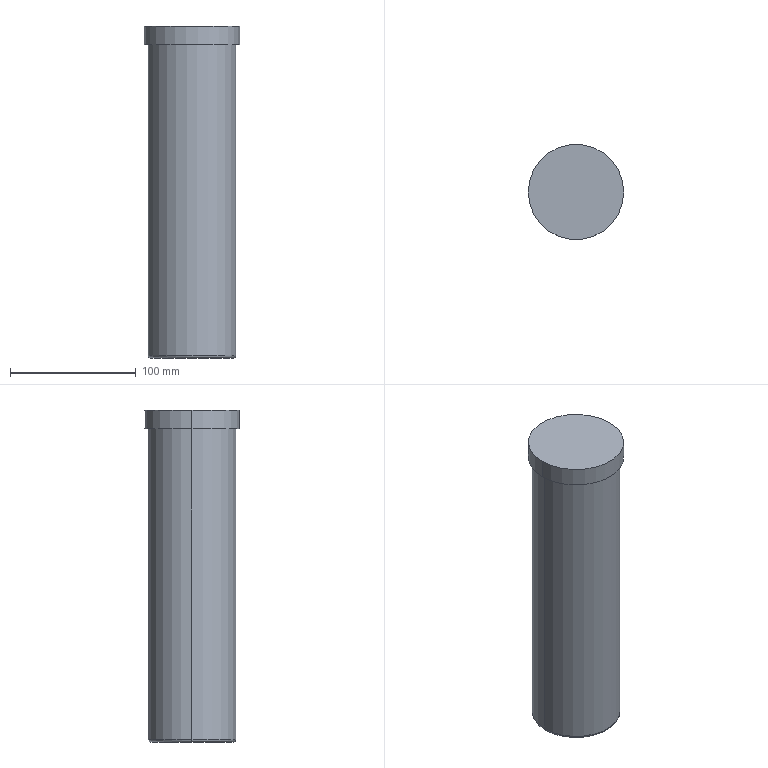Part | SolidWorks | features BaseBody 1 | 1 solid | 9 faces | box 76 x 76 x 264.5 mm | volume 1028049 mm3 | cylinder 4 | plane 3 | torus 2 | commonest cylinder face diameters 70 x2 76 x2
STEP:
#1=CARTESIAN_POINT('',(-378.,-275.,-94.));
#2=VERTEX_POINT('',#1);
#3=CARTESIAN_POINT('',(-312.,-275.,-94.));
#4=VERTEX_POINT('',#3);
#5=CARTESIAN_POINT('',(-345.,-275.,-94.));
#6=DIRECTION('',(0.,0.,-1.));
#7=DIRECTION('',(1.,0.,0.));
#8=AXIS2_PLACEMENT_3D('',#5,#6,#7);
#9=CIRCLE('',#8,33.);
#10=EDGE_CURVE('',#2,#4,#9,.T.);
#11=ORIENTED_EDGE('',*,*,#10,.F.);
#12=CARTESIAN_POINT('',(-380.,-275.,-92.));
#13=VERTEX_POINT('',#12);
#14=CARTESIAN_POINT('',(-378.,-275.,-92.));
#15=DIRECTION('',(0.,1.,0.));
#16=DIRECTION('',(-1.,0.,0.));
#17=AXIS2_PLACEMENT_3D('',#14,#15,#16);
#18=CIRCLE('',#17,2.);
#19=EDGE_CURVE('',#2,#13,#18,.T.);
#20=ORIENTED_EDGE('',*,*,#19,.T.);
#21=CARTESIAN_POINT('',(-310.,-275.,-92.));
#22=VERTEX_POINT('',#21);
#23=CARTESIAN_POINT('',(-345.,-275.,-92.));
#24=DIRECTION('',(0.,0.,1.));
#25=DIRECTION('',(1.,0.,0.));
#26=AXIS2_PLACEMENT_3D('',#23,#24,#25);
#27=CIRCLE('',#26,35.);
#28=EDGE_CURVE('',#22,#13,#27,.T.);
#29=ORIENTED_EDGE('',*,*,#28,.F.);
#30=CARTESIAN_POINT('',(-312.,-275.,-92.));
#31=DIRECTION('',(0.,-1.,0.));
#32=DIRECTION('',(0.,0.,-1.));
#33=AXIS2_PLACEMENT_3D('',#30,#31,#32);
#34=CIRCLE('',#33,2.);
#35=EDGE_CURVE('',#4,#22,#34,.T.);
#36=ORIENTED_EDGE('',*,*,#35,.F.);
#37=EDGE_LOOP('',(#11,#20,#29,#36));
#38=FACE_OUTER_BOUND('',#37,.T.);
#39=CARTESIAN_POINT('',(-345.,-275.,-92.));
#40=DIRECTION('',(0.,0.,1.));
#41=DIRECTION('',(1.,0.,0.));
#42=AXIS2_PLACEMENT_3D('',#39,#40,#41);
#43=TOROIDAL_SURFACE('',#42,33.,2.);
#44=ADVANCED_FACE('',(#38),#43,.T.);
#45=CARTESIAN_POINT('',(-383.,-275.,170.5));
#46=VERTEX_POINT('',#45);
#47=CARTESIAN_POINT('',(-307.,-275.,170.5));
#48=VERTEX_POINT('',#47);
#49=CARTESIAN_POINT('',(-345.,-275.,170.5));
#50=DIRECTION('',(0.,0.,-1.));
#51=DIRECTION('',(-1.,0.,0.));
#52=AXIS2_PLACEMENT_3D('',#49,#50,#51);
#53=CIRCLE('',#52,38.);
#54=EDGE_CURVE('',#46,#48,#53,.T.);
#55=ORIENTED_EDGE('',*,*,#54,.T.);
#56=CARTESIAN_POINT('',(-307.,-275.,155.5));
#57=VERTEX_POINT('',#56);
#58=CARTESIAN_POINT('',(-307.,-275.,170.5));
#59=DIRECTION('',(0.,0.,-1.));
#60=VECTOR('',#59,1000.);
#61=LINE('',#58,#60);
#62=EDGE_CURVE('',#48,#57,#61,.T.);
#63=ORIENTED_EDGE('',*,*,#62,.T.);
#64=CARTESIAN_POINT('',(-383.,-275.,155.5));
#65=VERTEX_POINT('',#64);
#66=CARTESIAN_POINT('',(-345.,-275.,155.5));
#67=DIRECTION('',(0.,0.,-1.));
#68=DIRECTION('',(-1.,0.,0.));
#69=AXIS2_PLACEMENT_3D('',#66,#67,#68);
#70=CIRCLE('',#69,38.);
#71=EDGE_CURVE('',#65,#57,#70,.T.);
#72=ORIENTED_EDGE('',*,*,#71,.F.);
#73=CARTESIAN_POINT('',(-383.,-275.,170.5));
#74=DIRECTION('',(0.,0.,-1.));
#75=VECTOR('',#74,1000.);
#76=LINE('',#73,#75);
#77=EDGE_CURVE('',#46,#65,#76,.T.);
#78=ORIENTED_EDGE('',*,*,#77,.F.);
#79=EDGE_LOOP('',(#55,#63,#72,#78));
#80=FACE_OUTER_BOUND('',#79,.T.);
#81=CARTESIAN_POINT('',(-345.,-275.,170.5));
#82=DIRECTION('',(0.,0.,-1.));
#83=DIRECTION('',(-1.,0.,0.));
#84=AXIS2_PLACEMENT_3D('',#81,#82,#83);
#85=CYLINDRICAL_SURFACE('',#84,38.);
#86=ADVANCED_FACE('',(#80),#85,.T.);
#87=CARTESIAN_POINT('',(-380.,-275.,155.5));
#88=VERTEX_POINT('',#87);
#89=CARTESIAN_POINT('',(-310.,-275.,155.5));
#90=VERTEX_POINT('',#89);
#91=CARTESIAN_POINT('',(-345.,-275.,155.5));
#92=DIRECTION('',(0.,0.,-1.));
#93=DIRECTION('',(1.,0.,0.));
#94=AXIS2_PLACEMENT_3D('',#91,#92,#93);
#95=CIRCLE('',#94,35.);
#96=EDGE_CURVE('',#88,#90,#95,.T.);
#97=ORIENTED_EDGE('',*,*,#96,.T.);
#98=CARTESIAN_POINT('',(-310.,-275.,170.5));
#99=DIRECTION('',(0.,0.,-1.));
#100=VECTOR('',#99,1000.);
#101=LINE('',#98,#100);
#102=EDGE_CURVE('',#90,#22,#101,.T.);
#103=ORIENTED_EDGE('',*,*,#102,.T.);
#104=ORIENTED_EDGE('',*,*,#28,.T.);
#105=CARTESIAN_POINT('',(-380.,-275.,170.5));
#106=DIRECTION('',(0.,0.,-1.));
#107=VECTOR('',#106,1000.);
#108=LINE('',#105,#107);
#109=EDGE_CURVE('',#88,#13,#108,.T.);
#110=ORIENTED_EDGE('',*,*,#109,.F.);
#111=EDGE_LOOP('',(#97,#103,#104,#110));
#112=FACE_OUTER_BOUND('',#111,.T.);
#113=CARTESIAN_POINT('',(-345.,-275.,170.5));
#114=DIRECTION('',(0.,0.,-1.));
#115=DIRECTION('',(-1.,0.,0.));
#116=AXIS2_PLACEMENT_3D('',#113,#114,#115);
#117=CYLINDRICAL_SURFACE('',#116,35.);
#118=ADVANCED_FACE('',(#112),#117,.T.);
#119=ORIENTED_EDGE('',*,*,#102,.F.);
#120=CARTESIAN_POINT('',(-345.,-275.,155.5));
#121=DIRECTION('',(0.,0.,-1.));
#122=DIRECTION('',(1.,0.,0.));
#123=AXIS2_PLACEMENT_3D('',#120,#121,#122);
#124=CIRCLE('',#123,35.);
#125=EDGE_CURVE('',#90,#88,#124,.T.);
#126=ORIENTED_EDGE('',*,*,#125,.T.);
#127=ORIENTED_EDGE('',*,*,#109,.T.);
#128=CARTESIAN_POINT('',(-345.,-275.,-92.));
#129=DIRECTION('',(0.,0.,1.));
#130=DIRECTION('',(1.,0.,0.));
#131=AXIS2_PLACEMENT_3D('',#128,#129,#130);
#132=CIRCLE('',#131,35.);
#133=EDGE_CURVE('',#13,#22,#132,.T.);
#134=ORIENTED_EDGE('',*,*,#133,.T.);
#135=EDGE_LOOP('',(#119,#126,#127,#134));
#136=FACE_OUTER_BOUND('',#135,.T.);
#137=CARTESIAN_POINT('',(-345.,-275.,170.5));
#138=DIRECTION('',(0.,0.,-1.));
#139=DIRECTION('',(-1.,0.,0.));
#140=AXIS2_PLACEMENT_3D('',#137,#138,#139);
#141=CYLINDRICAL_SURFACE('',#140,35.);
#142=ADVANCED_FACE('',(#136),#141,.T.);
#143=CARTESIAN_POINT('',(-345.,-275.,-94.));
#144=DIRECTION('',(0.,0.,-1.));
#145=DIRECTION('',(1.,0.,0.));
#146=AXIS2_PLACEMENT_3D('',#143,#144,#145);
#147=CIRCLE('',#146,33.);
#148=EDGE_CURVE('',#4,#2,#147,.T.);
#149=ORIENTED_EDGE('',*,*,#148,.T.);
#150=ORIENTED_EDGE('',*,*,#10,.T.);
#151=EDGE_LOOP('',(#149,#150));
#152=FACE_OUTER_BOUND('',#151,.T.);
#153=CARTESIAN_POINT('',(-345.,-275.,-94.));
#154=DIRECTION('',(0.,0.,1.));
#155=DIRECTION('',(1.,0.,0.));
#156=AXIS2_PLACEMENT_3D('',#153,#154,#155);
#157=PLANE('',#156);
#158=ADVANCED_FACE('',(#152),#157,.F.);
#159=ORIENTED_EDGE('',*,*,#62,.F.);
#160=CARTESIAN_POINT('',(-345.,-275.,170.5));
#161=DIRECTION('',(0.,0.,-1.));
#162=DIRECTION('',(-1.,0.,0.));
#163=AXIS2_PLACEMENT_3D('',#160,#161,#162);
#164=CIRCLE('',#163,38.);
#165=EDGE_CURVE('',#48,#46,#164,.T.);
#166=ORIENTED_EDGE('',*,*,#165,.T.);
#167=ORIENTED_EDGE('',*,*,#77,.T.);
#168=CARTESIAN_POINT('',(-345.,-275.,155.5));
#169=DIRECTION('',(0.,0.,-1.));
#170=DIRECTION('',(-1.,0.,0.));
#171=AXIS2_PLACEMENT_3D('',#168,#169,#170);
#172=CIRCLE('',#171,38.);
#173=EDGE_CURVE('',#57,#65,#172,.T.);
#174=ORIENTED_EDGE('',*,*,#173,.F.);
#175=EDGE_LOOP('',(#159,#166,#167,#174));
#176=FACE_OUTER_BOUND('',#175,.T.);
#177=CARTESIAN_POINT('',(-345.,-275.,170.5));
#178=DIRECTION('',(0.,0.,-1.));
#179=DIRECTION('',(-1.,0.,0.));
#180=AXIS2_PLACEMENT_3D('',#177,#178,#179);
#181=CYLINDRICAL_SURFACE('',#180,38.);
#182=ADVANCED_FACE('',(#176),#181,.T.);
#183=ORIENTED_EDGE('',*,*,#71,.T.);
#184=ORIENTED_EDGE('',*,*,#173,.T.);
#185=EDGE_LOOP('',(#183,#184));
#186=FACE_OUTER_BOUND('',#185,.T.);
#187=ORIENTED_EDGE('',*,*,#96,.F.);
#188=ORIENTED_EDGE('',*,*,#125,.F.);
#189=EDGE_LOOP('',(#187,#188));
#190=FACE_BOUND('',#189,.T.);
#191=CARTESIAN_POINT('',(-345.,-275.,155.5));
#192=DIRECTION('',(0.,0.,1.));
#193=DIRECTION('',(1.,0.,0.));
#194=AXIS2_PLACEMENT_3D('',#191,#192,#193);
#195=PLANE('',#194);
#196=ADVANCED_FACE('',(#186,#190),#195,.F.);
#197=ORIENTED_EDGE('',*,*,#54,.F.);
#198=ORIENTED_EDGE('',*,*,#165,.F.);
#199=EDGE_LOOP('',(#197,#198));
#200=FACE_OUTER_BOUND('',#199,.T.);
#201=CARTESIAN_POINT('',(-345.,-275.,170.5));
#202=DIRECTION('',(0.,0.,1.));
#203=DIRECTION('',(1.,0.,0.));
#204=AXIS2_PLACEMENT_3D('',#201,#202,#203);
#205=PLANE('',#204);
#206=ADVANCED_FACE('',(#200),#205,.T.);
#207=ORIENTED_EDGE('',*,*,#19,.F.);
#208=ORIENTED_EDGE('',*,*,#148,.F.);
#209=ORIENTED_EDGE('',*,*,#35,.T.);
#210=ORIENTED_EDGE('',*,*,#133,.F.);
#211=EDGE_LOOP('',(#207,#208,#209,#210));
#212=FACE_OUTER_BOUND('',#211,.T.);
#213=CARTESIAN_POINT('',(-345.,-275.,-92.));
#214=DIRECTION('',(0.,0.,1.));
#215=DIRECTION('',(1.,0.,0.));
#216=AXIS2_PLACEMENT_3D('',#213,#214,#215);
#217=TOROIDAL_SURFACE('',#216,33.,2.);
#218=ADVANCED_FACE('',(#212),#217,.T.);
#219=CLOSED_SHELL('',(#44,#86,#118,#142,#158,#182,#196,#206,#218));
#220=MANIFOLD_SOLID_BREP('',#219);
#221=CARTESIAN_POINT('',(0.,0.,0.));
#222=DIRECTION('',(0.,0.,1.));
#223=DIRECTION('',(1.,0.,0.));
#224=AXIS2_PLACEMENT_3D('',#221,#222,#223);
#225=(LENGTH_UNIT()NAMED_UNIT(*)SI_UNIT(.MILLI.,.METRE.));
#226=UNCERTAINTY_MEASURE_WITH_UNIT(LENGTH_MEASURE(0.00001),#225,'','');
#227=(NAMED_UNIT(*)PLANE_ANGLE_UNIT()SI_UNIT($,.RADIAN.));
#228=(NAMED_UNIT(*)SI_UNIT($,.STERADIAN.)SOLID_ANGLE_UNIT());
#229=(GEOMETRIC_REPRESENTATION_CONTEXT(3)GLOBAL_UNCERTAINTY_ASSIGNED_CONTEXT((#226))GLOBAL_UNIT_ASSIGNED_CONTEXT((#225,#227,#228))REPRESENTATION_CONTEXT('',''));
#230=ADVANCED_BREP_SHAPE_REPRESENTATION('',(#220,#224),#229);